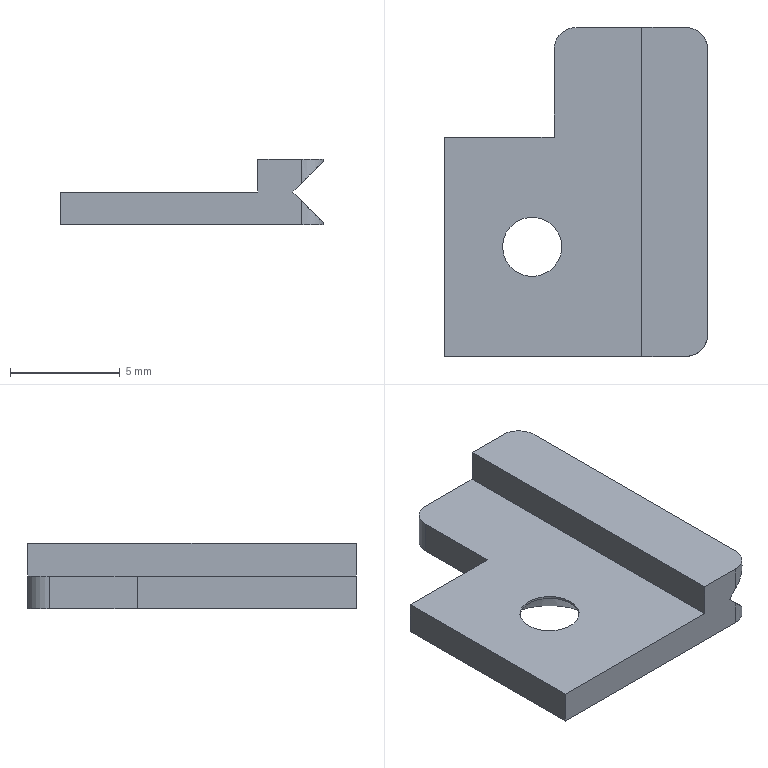Part | NX | features BREP 1 | 1 solid | 22 faces | box 12 x 15 x 3 mm | volume 250.226 mm3 | plane 13 | cylinder 7 | cone 2 | commonest cylinder face diameters 2 x5 2.7 x2
STEP:
#1=CARTESIAN_POINT('',(3.,7.5,3.));
#2=VERTEX_POINT('',#1);
#3=CARTESIAN_POINT('',(3.,7.5,1.5));
#4=VERTEX_POINT('',#3);
#5=CARTESIAN_POINT('',(3.,7.5,3.));
#6=DIRECTION('',(0.,0.,-1.));
#7=VECTOR('',#6,1000.);
#8=LINE('',#5,#7);
#9=EDGE_CURVE('',#2,#4,#8,.T.);
#10=ORIENTED_EDGE('',*,*,#9,.T.);
#11=CARTESIAN_POINT('',(3.,-7.5,1.5));
#12=VERTEX_POINT('',#11);
#13=CARTESIAN_POINT('',(3.,-7.5,1.5));
#14=DIRECTION('',(0.,1.,0.));
#15=VECTOR('',#14,1000.);
#16=LINE('',#13,#15);
#17=EDGE_CURVE('',#12,#4,#16,.T.);
#18=ORIENTED_EDGE('',*,*,#17,.F.);
#19=CARTESIAN_POINT('',(3.,-7.5,3.));
#20=VERTEX_POINT('',#19);
#21=CARTESIAN_POINT('',(3.,-7.5,3.));
#22=DIRECTION('',(0.,0.,-1.));
#23=VECTOR('',#22,1000.);
#24=LINE('',#21,#23);
#25=EDGE_CURVE('',#20,#12,#24,.T.);
#26=ORIENTED_EDGE('',*,*,#25,.F.);
#27=CARTESIAN_POINT('',(3.,-7.5,3.));
#28=DIRECTION('',(0.,1.,0.));
#29=VECTOR('',#28,1000.);
#30=LINE('',#27,#29);
#31=EDGE_CURVE('',#20,#2,#30,.T.);
#32=ORIENTED_EDGE('',*,*,#31,.T.);
#33=EDGE_LOOP('',(#10,#18,#26,#32));
#34=FACE_BOUND('',#33,.T.);
#35=CARTESIAN_POINT('',(3.,-7.5,3.));
#36=DIRECTION('',(1.,0.,0.));
#37=DIRECTION('',(0.,0.,-1.));
#38=AXIS2_PLACEMENT_3D('',#35,#36,#37);
#39=PLANE('',#38);
#40=ADVANCED_FACE('',(#34),#39,.F.);
#41=CARTESIAN_POINT('',(-6.,-7.5,1.5));
#42=VERTEX_POINT('',#41);
#43=CARTESIAN_POINT('',(-6.,2.5,1.5));
#44=VERTEX_POINT('',#43);
#45=CARTESIAN_POINT('',(-6.,-7.5,1.5));
#46=DIRECTION('',(0.,1.,0.));
#47=VECTOR('',#46,1000.);
#48=LINE('',#45,#47);
#49=EDGE_CURVE('',#42,#44,#48,.T.);
#50=ORIENTED_EDGE('',*,*,#49,.F.);
#51=CARTESIAN_POINT('',(-6.,-7.5,1.5));
#52=DIRECTION('',(-1.,0.,0.));
#53=VECTOR('',#52,1000.);
#54=LINE('',#51,#53);
#55=EDGE_CURVE('',#12,#42,#54,.T.);
#56=ORIENTED_EDGE('',*,*,#55,.F.);
#57=ORIENTED_EDGE('',*,*,#17,.T.);
#58=CARTESIAN_POINT('',(0.,7.5,1.5));
#59=VERTEX_POINT('',#58);
#60=CARTESIAN_POINT('',(-6.,7.5,1.5));
#61=DIRECTION('',(-1.,0.,0.));
#62=VECTOR('',#61,1000.);
#63=LINE('',#60,#62);
#64=EDGE_CURVE('',#4,#59,#63,.T.);
#65=ORIENTED_EDGE('',*,*,#64,.T.);
#66=CARTESIAN_POINT('',(-1.,6.5,1.5));
#67=VERTEX_POINT('',#66);
#68=CARTESIAN_POINT('',(0.,6.5,1.5));
#69=DIRECTION('',(0.,0.,1.));
#70=DIRECTION('',(-1.,0.,0.));
#71=AXIS2_PLACEMENT_3D('',#68,#69,#70);
#72=CIRCLE('',#71,1.);
#73=EDGE_CURVE('',#59,#67,#72,.T.);
#74=ORIENTED_EDGE('',*,*,#73,.T.);
#75=CARTESIAN_POINT('',(-1.,2.5,1.5));
#76=VERTEX_POINT('',#75);
#77=CARTESIAN_POINT('',(-1.,7.5,1.5));
#78=DIRECTION('',(0.,1.,0.));
#79=VECTOR('',#78,1000.);
#80=LINE('',#77,#79);
#81=EDGE_CURVE('',#76,#67,#80,.T.);
#82=ORIENTED_EDGE('',*,*,#81,.F.);
#83=CARTESIAN_POINT('',(-6.,2.5,1.5));
#84=DIRECTION('',(1.,0.,0.));
#85=VECTOR('',#84,1000.);
#86=LINE('',#83,#85);
#87=EDGE_CURVE('',#44,#76,#86,.T.);
#88=ORIENTED_EDGE('',*,*,#87,.F.);
#89=EDGE_LOOP('',(#50,#56,#57,#65,#74,#82,#88));
#90=FACE_BOUND('',#89,.T.);
#91=CARTESIAN_POINT('',(-3.35,-2.5,1.5));
#92=VERTEX_POINT('',#91);
#93=CARTESIAN_POINT('',(-0.65,-2.5,1.5));
#94=VERTEX_POINT('',#93);
#95=CARTESIAN_POINT('',(-2.,-2.5,1.5));
#96=DIRECTION('',(0.,0.,1.));
#97=DIRECTION('',(-1.,0.,0.));
#98=AXIS2_PLACEMENT_3D('',#95,#96,#97);
#99=CIRCLE('',#98,1.35);
#100=EDGE_CURVE('',#92,#94,#99,.T.);
#101=ORIENTED_EDGE('',*,*,#100,.F.);
#102=CARTESIAN_POINT('',(-2.,-2.5,1.5));
#103=DIRECTION('',(0.,0.,1.));
#104=DIRECTION('',(-1.,0.,0.));
#105=AXIS2_PLACEMENT_3D('',#102,#103,#104);
#106=CIRCLE('',#105,1.35);
#107=EDGE_CURVE('',#94,#92,#106,.T.);
#108=ORIENTED_EDGE('',*,*,#107,.F.);
#109=EDGE_LOOP('',(#101,#108));
#110=FACE_BOUND('',#109,.T.);
#111=CARTESIAN_POINT('',(-6.,-7.5,1.5));
#112=DIRECTION('',(0.,0.,-1.));
#113=DIRECTION('',(-1.,0.,0.));
#114=AXIS2_PLACEMENT_3D('',#111,#112,#113);
#115=PLANE('',#114);
#116=ADVANCED_FACE('',(#90,#110),#115,.F.);
#117=CARTESIAN_POINT('',(-0.65,-2.5,1.4));
#118=VERTEX_POINT('',#117);
#119=CARTESIAN_POINT('',(0.75,-2.5,0.));
#120=VERTEX_POINT('',#119);
#121=CARTESIAN_POINT('',(0.75,-2.5,0.));
#122=DIRECTION('',(0.7071,0.,-0.7071));
#123=VECTOR('',#122,1000.);
#124=LINE('',#121,#123);
#125=EDGE_CURVE('',#118,#120,#124,.T.);
#126=ORIENTED_EDGE('',*,*,#125,.F.);
#127=CARTESIAN_POINT('',(-3.35,-2.5,1.4));
#128=VERTEX_POINT('',#127);
#129=CARTESIAN_POINT('',(-2.,-2.5,1.4));
#130=DIRECTION('',(0.,0.,-1.));
#131=DIRECTION('',(-1.,0.,0.));
#132=AXIS2_PLACEMENT_3D('',#129,#130,#131);
#133=CIRCLE('',#132,1.35);
#134=EDGE_CURVE('',#128,#118,#133,.T.);
#135=ORIENTED_EDGE('',*,*,#134,.F.);
#136=CARTESIAN_POINT('',(-4.75,-2.5,0.));
#137=VERTEX_POINT('',#136);
#138=CARTESIAN_POINT('',(-4.75,-2.5,0.));
#139=DIRECTION('',(-0.7071,0.,-0.7071));
#140=VECTOR('',#139,1000.);
#141=LINE('',#138,#140);
#142=EDGE_CURVE('',#128,#137,#141,.T.);
#143=ORIENTED_EDGE('',*,*,#142,.T.);
#144=CARTESIAN_POINT('',(-2.,-2.5,0.));
#145=DIRECTION('',(0.,0.,-1.));
#146=DIRECTION('',(-1.,0.,0.));
#147=AXIS2_PLACEMENT_3D('',#144,#145,#146);
#148=CIRCLE('',#147,2.75);
#149=EDGE_CURVE('',#137,#120,#148,.T.);
#150=ORIENTED_EDGE('',*,*,#149,.T.);
#151=EDGE_LOOP('',(#126,#135,#143,#150));
#152=FACE_BOUND('',#151,.T.);
#153=CARTESIAN_POINT('',(-2.,-2.5,0.));
#154=DIRECTION('',(0.,0.,-1.));
#155=DIRECTION('',(-1.,0.,0.));
#156=AXIS2_PLACEMENT_3D('',#153,#154,#155);
#157=CONICAL_SURFACE('',#156,2.75,0.7854);
#158=ADVANCED_FACE('',(#152),#157,.F.);
#159=CARTESIAN_POINT('',(-0.65,-2.5,0.));
#160=DIRECTION('',(0.,0.,-1.));
#161=VECTOR('',#160,1000.);
#162=LINE('',#159,#161);
#163=EDGE_CURVE('',#94,#118,#162,.T.);
#164=ORIENTED_EDGE('',*,*,#163,.F.);
#165=ORIENTED_EDGE('',*,*,#107,.T.);
#166=CARTESIAN_POINT('',(-3.35,-2.5,0.));
#167=DIRECTION('',(0.,0.,-1.));
#168=VECTOR('',#167,1000.);
#169=LINE('',#166,#168);
#170=EDGE_CURVE('',#92,#128,#169,.T.);
#171=ORIENTED_EDGE('',*,*,#170,.T.);
#172=ORIENTED_EDGE('',*,*,#134,.T.);
#173=EDGE_LOOP('',(#164,#165,#171,#172));
#174=FACE_BOUND('',#173,.T.);
#175=CARTESIAN_POINT('',(-2.,-2.5,0.));
#176=DIRECTION('',(0.,0.,-1.));
#177=DIRECTION('',(-1.,0.,0.));
#178=AXIS2_PLACEMENT_3D('',#175,#176,#177);
#179=CYLINDRICAL_SURFACE('',#178,1.35);
#180=ADVANCED_FACE('',(#174),#179,.F.);
#181=CARTESIAN_POINT('',(5.,-7.5,1.1));
#182=VERTEX_POINT('',#181);
#183=CARTESIAN_POINT('',(6.,-6.5,0.1));
#184=VERTEX_POINT('',#183);
#185=CARTESIAN_POINT('',(5.,-7.5,1.1));
#186=CARTESIAN_POINT('',(5.586,-7.5,0.5142));
#187=CARTESIAN_POINT('',(6.,-7.086,0.1));
#188=CARTESIAN_POINT('',(6.,-6.5,0.1));
#189=(BOUNDED_CURVE()B_SPLINE_CURVE(3,(#185,#186,#187,#188),.UNSPECIFIED.,.F.,.F.)B_SPLINE_CURVE_WITH_KNOTS((4,4),(4.712,6.283),.UNSPECIFIED.)CURVE()GEOMETRIC_REPRESENTATION_ITEM()RATIONAL_B_SPLINE_CURVE((1.,0.8047,0.8047,1.))REPRESENTATION_ITEM(''));
#190=EDGE_CURVE('',#182,#184,#189,.T.);
#191=ORIENTED_EDGE('',*,*,#190,.T.);
#192=CARTESIAN_POINT('',(6.,6.5,0.1));
#193=VERTEX_POINT('',#192);
#194=CARTESIAN_POINT('',(6.,-12.5,0.1));
#195=DIRECTION('',(0.,1.,0.));
#196=VECTOR('',#195,1000.);
#197=LINE('',#194,#196);
#198=EDGE_CURVE('',#184,#193,#197,.T.);
#199=ORIENTED_EDGE('',*,*,#198,.T.);
#200=CARTESIAN_POINT('',(5.,7.5,1.1));
#201=VERTEX_POINT('',#200);
#202=CARTESIAN_POINT('',(6.,6.5,0.1));
#203=CARTESIAN_POINT('',(6.,7.086,0.1));
#204=CARTESIAN_POINT('',(5.586,7.5,0.5142));
#205=CARTESIAN_POINT('',(5.,7.5,1.1));
#206=(BOUNDED_CURVE()B_SPLINE_CURVE(3,(#202,#203,#204,#205),.UNSPECIFIED.,.F.,.F.)B_SPLINE_CURVE_WITH_KNOTS((4,4),(0.,1.571),.UNSPECIFIED.)CURVE()GEOMETRIC_REPRESENTATION_ITEM()RATIONAL_B_SPLINE_CURVE((1.,0.8047,0.8047,1.))REPRESENTATION_ITEM(''));
#207=EDGE_CURVE('',#193,#201,#206,.T.);
#208=ORIENTED_EDGE('',*,*,#207,.T.);
#209=CARTESIAN_POINT('',(4.6,7.5,1.5));
#210=VERTEX_POINT('',#209);
#211=CARTESIAN_POINT('',(4.6,7.5,1.5));
#212=DIRECTION('',(-0.7071,0.,0.7071));
#213=VECTOR('',#212,1000.);
#214=LINE('',#211,#213);
#215=EDGE_CURVE('',#201,#210,#214,.T.);
#216=ORIENTED_EDGE('',*,*,#215,.T.);
#217=CARTESIAN_POINT('',(4.6,-7.5,1.5));
#218=VERTEX_POINT('',#217);
#219=CARTESIAN_POINT('',(4.6,-12.5,1.5));
#220=DIRECTION('',(0.,1.,0.));
#221=VECTOR('',#220,1000.);
#222=LINE('',#219,#221);
#223=EDGE_CURVE('',#218,#210,#222,.T.);
#224=ORIENTED_EDGE('',*,*,#223,.F.);
#225=CARTESIAN_POINT('',(-1.45,-7.5,7.55));
#226=DIRECTION('',(-0.7071,0.,0.7071));
#227=VECTOR('',#226,1000.);
#228=LINE('',#225,#227);
#229=EDGE_CURVE('',#182,#218,#228,.T.);
#230=ORIENTED_EDGE('',*,*,#229,.F.);
#231=EDGE_LOOP('',(#191,#199,#208,#216,#224,#230));
#232=FACE_BOUND('',#231,.T.);
#233=CARTESIAN_POINT('',(4.6,-12.5,1.5));
#234=DIRECTION('',(-0.7071,0.,-0.7071));
#235=DIRECTION('',(-0.7071,0.,0.7071));
#236=AXIS2_PLACEMENT_3D('',#233,#234,#235);
#237=PLANE('',#236);
#238=ADVANCED_FACE('',(#232),#237,.F.);
#239=ORIENTED_EDGE('',*,*,#223,.T.);
#240=CARTESIAN_POINT('',(5.,7.5,1.9));
#241=VERTEX_POINT('',#240);
#242=CARTESIAN_POINT('',(6.,7.5,2.9));
#243=DIRECTION('',(0.7071,0.,0.7071));
#244=VECTOR('',#243,1000.);
#245=LINE('',#242,#244);
#246=EDGE_CURVE('',#210,#241,#245,.T.);
#247=ORIENTED_EDGE('',*,*,#246,.T.);
#248=CARTESIAN_POINT('',(6.,6.5,2.9));
#249=VERTEX_POINT('',#248);
#250=CARTESIAN_POINT('',(5.,7.5,1.9));
#251=CARTESIAN_POINT('',(5.586,7.5,2.486));
#252=CARTESIAN_POINT('',(6.,7.086,2.9));
#253=CARTESIAN_POINT('',(6.,6.5,2.9));
#254=(BOUNDED_CURVE()B_SPLINE_CURVE(3,(#250,#251,#252,#253),.UNSPECIFIED.,.F.,.F.)B_SPLINE_CURVE_WITH_KNOTS((4,4),(1.571,3.142),.UNSPECIFIED.)CURVE()GEOMETRIC_REPRESENTATION_ITEM()RATIONAL_B_SPLINE_CURVE((1.,0.8047,0.8047,1.))REPRESENTATION_ITEM(''));
#255=EDGE_CURVE('',#241,#249,#254,.T.);
#256=ORIENTED_EDGE('',*,*,#255,.T.);
#257=CARTESIAN_POINT('',(6.,-6.5,2.9));
#258=VERTEX_POINT('',#257);
#259=CARTESIAN_POINT('',(6.,-12.5,2.9));
#260=DIRECTION('',(0.,1.,0.));
#261=VECTOR('',#260,1000.);
#262=LINE('',#259,#261);
#263=EDGE_CURVE('',#258,#249,#262,.T.);
#264=ORIENTED_EDGE('',*,*,#263,.F.);
#265=CARTESIAN_POINT('',(5.,-7.5,1.9));
#266=VERTEX_POINT('',#265);
#267=CARTESIAN_POINT('',(6.,-6.5,2.9));
#268=CARTESIAN_POINT('',(6.,-7.086,2.9));
#269=CARTESIAN_POINT('',(5.586,-7.5,2.486));
#270=CARTESIAN_POINT('',(5.,-7.5,1.9));
#271=(BOUNDED_CURVE()B_SPLINE_CURVE(3,(#267,#268,#269,#270),.UNSPECIFIED.,.F.,.F.)B_SPLINE_CURVE_WITH_KNOTS((4,4),(3.142,4.712),.UNSPECIFIED.)CURVE()GEOMETRIC_REPRESENTATION_ITEM()RATIONAL_B_SPLINE_CURVE((1.,0.8047,0.8047,1.))REPRESENTATION_ITEM(''));
#272=EDGE_CURVE('',#258,#266,#271,.T.);
#273=ORIENTED_EDGE('',*,*,#272,.T.);
#274=CARTESIAN_POINT('',(0.05,-7.5,-3.05));
#275=DIRECTION('',(0.7071,0.,0.7071));
#276=VECTOR('',#275,1000.);
#277=LINE('',#274,#276);
#278=EDGE_CURVE('',#218,#266,#277,.T.);
#279=ORIENTED_EDGE('',*,*,#278,.F.);
#280=EDGE_LOOP('',(#239,#247,#256,#264,#273,#279));
#281=FACE_BOUND('',#280,.T.);
#282=CARTESIAN_POINT('',(6.,-12.5,2.9));
#283=DIRECTION('',(-0.7071,0.,0.7071));
#284=DIRECTION('',(0.7071,0.,0.7071));
#285=AXIS2_PLACEMENT_3D('',#282,#283,#284);
#286=PLANE('',#285);
#287=ADVANCED_FACE('',(#281),#286,.F.);
#288=ORIENTED_EDGE('',*,*,#207,.F.);
#289=CARTESIAN_POINT('',(6.,6.5,0.));
#290=VERTEX_POINT('',#289);
#291=CARTESIAN_POINT('',(6.,6.5,3.));
#292=DIRECTION('',(0.,0.,1.));
#293=VECTOR('',#292,1000.);
#294=LINE('',#291,#293);
#295=EDGE_CURVE('',#290,#193,#294,.T.);
#296=ORIENTED_EDGE('',*,*,#295,.F.);
#297=CARTESIAN_POINT('',(5.,7.5,0.));
#298=VERTEX_POINT('',#297);
#299=CARTESIAN_POINT('',(5.,6.5,0.));
#300=DIRECTION('',(0.,0.,-1.));
#301=DIRECTION('',(-1.,0.,0.));
#302=AXIS2_PLACEMENT_3D('',#299,#300,#301);
#303=CIRCLE('',#302,1.);
#304=EDGE_CURVE('',#298,#290,#303,.T.);
#305=ORIENTED_EDGE('',*,*,#304,.F.);
#306=CARTESIAN_POINT('',(5.,7.5,3.));
#307=DIRECTION('',(0.,0.,-1.));
#308=VECTOR('',#307,1000.);
#309=LINE('',#306,#308);
#310=EDGE_CURVE('',#201,#298,#309,.T.);
#311=ORIENTED_EDGE('',*,*,#310,.F.);
#312=EDGE_LOOP('',(#288,#296,#305,#311));
#313=FACE_BOUND('',#312,.T.);
#314=CARTESIAN_POINT('',(5.,6.5,3.));
#315=DIRECTION('',(0.,0.,-1.));
#316=DIRECTION('',(-1.,0.,0.));
#317=AXIS2_PLACEMENT_3D('',#314,#315,#316);
#318=CYLINDRICAL_SURFACE('',#317,1.);
#319=ADVANCED_FACE('',(#313),#318,.T.);
#320=ORIENTED_EDGE('',*,*,#190,.F.);
#321=CARTESIAN_POINT('',(5.,-7.5,0.));
#322=VERTEX_POINT('',#321);
#323=CARTESIAN_POINT('',(5.,-7.5,3.));
#324=DIRECTION('',(0.,0.,1.));
#325=VECTOR('',#324,1000.);
#326=LINE('',#323,#325);
#327=EDGE_CURVE('',#322,#182,#326,.T.);
#328=ORIENTED_EDGE('',*,*,#327,.F.);
#329=CARTESIAN_POINT('',(6.,-6.5,0.));
#330=VERTEX_POINT('',#329);
#331=CARTESIAN_POINT('',(5.,-6.5,0.));
#332=DIRECTION('',(0.,0.,-1.));
#333=DIRECTION('',(-1.,0.,0.));
#334=AXIS2_PLACEMENT_3D('',#331,#332,#333);
#335=CIRCLE('',#334,1.);
#336=EDGE_CURVE('',#330,#322,#335,.T.);
#337=ORIENTED_EDGE('',*,*,#336,.F.);
#338=CARTESIAN_POINT('',(6.,-6.5,3.));
#339=DIRECTION('',(0.,0.,-1.));
#340=VECTOR('',#339,1000.);
#341=LINE('',#338,#340);
#342=EDGE_CURVE('',#184,#330,#341,.T.);
#343=ORIENTED_EDGE('',*,*,#342,.F.);
#344=EDGE_LOOP('',(#320,#328,#337,#343));
#345=FACE_BOUND('',#344,.T.);
#346=CARTESIAN_POINT('',(5.,-6.5,3.));
#347=DIRECTION('',(0.,0.,-1.));
#348=DIRECTION('',(-1.,0.,0.));
#349=AXIS2_PLACEMENT_3D('',#346,#347,#348);
#350=CYLINDRICAL_SURFACE('',#349,1.);
#351=ADVANCED_FACE('',(#345),#350,.T.);
#352=ORIENTED_EDGE('',*,*,#73,.F.);
#353=CARTESIAN_POINT('',(0.,7.5,0.));
#354=VERTEX_POINT('',#353);
#355=CARTESIAN_POINT('',(0.,7.5,3.));
#356=DIRECTION('',(0.,0.,1.));
#357=VECTOR('',#356,1000.);
#358=LINE('',#355,#357);
#359=EDGE_CURVE('',#354,#59,#358,.T.);
#360=ORIENTED_EDGE('',*,*,#359,.F.);
#361=CARTESIAN_POINT('',(-1.,6.5,0.));
#362=VERTEX_POINT('',#361);
#363=CARTESIAN_POINT('',(0.,6.5,0.));
#364=DIRECTION('',(0.,0.,-1.));
#365=DIRECTION('',(-1.,0.,0.));
#366=AXIS2_PLACEMENT_3D('',#363,#364,#365);
#367=CIRCLE('',#366,1.);
#368=EDGE_CURVE('',#362,#354,#367,.T.);
#369=ORIENTED_EDGE('',*,*,#368,.F.);
#370=CARTESIAN_POINT('',(-1.,6.5,3.));
#371=DIRECTION('',(0.,0.,-1.));
#372=VECTOR('',#371,1000.);
#373=LINE('',#370,#372);
#374=EDGE_CURVE('',#67,#362,#373,.T.);
#375=ORIENTED_EDGE('',*,*,#374,.F.);
#376=EDGE_LOOP('',(#352,#360,#369,#375));
#377=FACE_BOUND('',#376,.T.);
#378=CARTESIAN_POINT('',(0.,6.5,3.));
#379=DIRECTION('',(0.,0.,-1.));
#380=DIRECTION('',(-1.,0.,0.));
#381=AXIS2_PLACEMENT_3D('',#378,#379,#380);
#382=CYLINDRICAL_SURFACE('',#381,1.);
#383=ADVANCED_FACE('',(#377),#382,.T.);
#384=CARTESIAN_POINT('',(-1.,2.5,0.));
#385=VERTEX_POINT('',#384);
#386=CARTESIAN_POINT('',(-1.,2.5,3.));
#387=DIRECTION('',(0.,0.,-1.));
#388=VECTOR('',#387,1000.);
#389=LINE('',#386,#388);
#390=EDGE_CURVE('',#76,#385,#389,.T.);
#391=ORIENTED_EDGE('',*,*,#390,.F.);
#392=ORIENTED_EDGE('',*,*,#81,.T.);
#393=ORIENTED_EDGE('',*,*,#374,.T.);
#394=CARTESIAN_POINT('',(-1.,7.5,0.));
#395=DIRECTION('',(0.,-1.,0.));
#396=VECTOR('',#395,1000.);
#397=LINE('',#394,#396);
#398=EDGE_CURVE('',#362,#385,#397,.T.);
#399=ORIENTED_EDGE('',*,*,#398,.T.);
#400=EDGE_LOOP('',(#391,#392,#393,#399));
#401=FACE_BOUND('',#400,.T.);
#402=CARTESIAN_POINT('',(-1.,7.5,3.));
#403=DIRECTION('',(1.,0.,0.));
#404=DIRECTION('',(0.,1.,0.));
#405=AXIS2_PLACEMENT_3D('',#402,#403,#404);
#406=PLANE('',#405);
#407=ADVANCED_FACE('',(#401),#406,.F.);
#408=CARTESIAN_POINT('',(-6.,2.5,0.));
#409=VERTEX_POINT('',#408);
#410=CARTESIAN_POINT('',(-6.,2.5,3.));
#411=DIRECTION('',(0.,0.,-1.));
#412=VECTOR('',#411,1000.);
#413=LINE('',#410,#412);
#414=EDGE_CURVE('',#44,#409,#413,.T.);
#415=ORIENTED_EDGE('',*,*,#414,.F.);
#416=ORIENTED_EDGE('',*,*,#87,.T.);
#417=ORIENTED_EDGE('',*,*,#390,.T.);
#418=CARTESIAN_POINT('',(-6.,2.5,0.));
#419=DIRECTION('',(-1.,0.,0.));
#420=VECTOR('',#419,1000.);
#421=LINE('',#418,#420);
#422=EDGE_CURVE('',#385,#409,#421,.T.);
#423=ORIENTED_EDGE('',*,*,#422,.T.);
#424=EDGE_LOOP('',(#415,#416,#417,#423));
#425=FACE_BOUND('',#424,.T.);
#426=CARTESIAN_POINT('',(-6.,2.5,3.));
#427=DIRECTION('',(0.,-1.,0.));
#428=DIRECTION('',(1.,0.,0.));
#429=AXIS2_PLACEMENT_3D('',#426,#427,#428);
#430=PLANE('',#429);
#431=ADVANCED_FACE('',(#425),#430,.F.);
#432=ORIENTED_EDGE('',*,*,#398,.F.);
#433=ORIENTED_EDGE('',*,*,#368,.T.);
#434=CARTESIAN_POINT('',(-6.,7.5,0.));
#435=DIRECTION('',(-1.,0.,0.));
#436=VECTOR('',#435,1000.);
#437=LINE('',#434,#436);
#438=EDGE_CURVE('',#298,#354,#437,.T.);
#439=ORIENTED_EDGE('',*,*,#438,.F.);
#440=ORIENTED_EDGE('',*,*,#304,.T.);
#441=CARTESIAN_POINT('',(6.,-7.5,0.));
#442=DIRECTION('',(0.,1.,0.));
#443=VECTOR('',#442,1000.);
#444=LINE('',#441,#443);
#445=EDGE_CURVE('',#330,#290,#444,.T.);
#446=ORIENTED_EDGE('',*,*,#445,.F.);
#447=ORIENTED_EDGE('',*,*,#336,.T.);
#448=CARTESIAN_POINT('',(-6.,-7.5,0.));
#449=VERTEX_POINT('',#448);
#450=CARTESIAN_POINT('',(-6.,-7.5,0.));
#451=DIRECTION('',(1.,0.,0.));
#452=VECTOR('',#451,1000.);
#453=LINE('',#450,#452);
#454=EDGE_CURVE('',#449,#322,#453,.T.);
#455=ORIENTED_EDGE('',*,*,#454,.F.);
#456=CARTESIAN_POINT('',(-6.,-7.5,0.));
#457=DIRECTION('',(0.,-1.,0.));
#458=VECTOR('',#457,1000.);
#459=LINE('',#456,#458);
#460=EDGE_CURVE('',#409,#449,#459,.T.);
#461=ORIENTED_EDGE('',*,*,#460,.F.);
#462=ORIENTED_EDGE('',*,*,#422,.F.);
#463=EDGE_LOOP('',(#432,#433,#439,#440,#446,#447,#455,#461,#462));
#464=FACE_BOUND('',#463,.T.);
#465=ORIENTED_EDGE('',*,*,#149,.F.);
#466=CARTESIAN_POINT('',(-2.,-2.5,0.));
#467=DIRECTION('',(0.,0.,-1.));
#468=DIRECTION('',(-1.,0.,0.));
#469=AXIS2_PLACEMENT_3D('',#466,#467,#468);
#470=CIRCLE('',#469,2.75);
#471=EDGE_CURVE('',#120,#137,#470,.T.);
#472=ORIENTED_EDGE('',*,*,#471,.F.);
#473=EDGE_LOOP('',(#465,#472));
#474=FACE_BOUND('',#473,.T.);
#475=CARTESIAN_POINT('',(0.,0.,0.));
#476=DIRECTION('',(0.,0.,-1.));
#477=DIRECTION('',(-1.,0.,0.));
#478=AXIS2_PLACEMENT_3D('',#475,#476,#477);
#479=PLANE('',#478);
#480=ADVANCED_FACE('',(#464,#474),#479,.T.);
#481=CARTESIAN_POINT('',(5.,7.5,3.));
#482=VERTEX_POINT('',#481);
#483=CARTESIAN_POINT('',(-6.,7.5,3.));
#484=DIRECTION('',(-1.,0.,0.));
#485=VECTOR('',#484,1000.);
#486=LINE('',#483,#485);
#487=EDGE_CURVE('',#482,#2,#486,.T.);
#488=ORIENTED_EDGE('',*,*,#487,.T.);
#489=ORIENTED_EDGE('',*,*,#31,.F.);
#490=CARTESIAN_POINT('',(5.,-7.5,3.));
#491=VERTEX_POINT('',#490);
#492=CARTESIAN_POINT('',(-6.,-7.5,3.));
#493=DIRECTION('',(1.,0.,0.));
#494=VECTOR('',#493,1000.);
#495=LINE('',#492,#494);
#496=EDGE_CURVE('',#20,#491,#495,.T.);
#497=ORIENTED_EDGE('',*,*,#496,.T.);
#498=CARTESIAN_POINT('',(6.,-6.5,3.));
#499=VERTEX_POINT('',#498);
#500=CARTESIAN_POINT('',(5.,-6.5,3.));
#501=DIRECTION('',(0.,0.,1.));
#502=DIRECTION('',(-1.,0.,0.));
#503=AXIS2_PLACEMENT_3D('',#500,#501,#502);
#504=CIRCLE('',#503,1.);
#505=EDGE_CURVE('',#491,#499,#504,.T.);
#506=ORIENTED_EDGE('',*,*,#505,.T.);
#507=CARTESIAN_POINT('',(6.,6.5,3.));
#508=VERTEX_POINT('',#507);
#509=CARTESIAN_POINT('',(6.,-7.5,3.));
#510=DIRECTION('',(0.,1.,0.));
#511=VECTOR('',#510,1000.);
#512=LINE('',#509,#511);
#513=EDGE_CURVE('',#499,#508,#512,.T.);
#514=ORIENTED_EDGE('',*,*,#513,.T.);
#515=CARTESIAN_POINT('',(5.,6.5,3.));
#516=DIRECTION('',(0.,0.,1.));
#517=DIRECTION('',(-1.,0.,0.));
#518=AXIS2_PLACEMENT_3D('',#515,#516,#517);
#519=CIRCLE('',#518,1.);
#520=EDGE_CURVE('',#508,#482,#519,.T.);
#521=ORIENTED_EDGE('',*,*,#520,.T.);
#522=EDGE_LOOP('',(#488,#489,#497,#506,#514,#521));
#523=FACE_BOUND('',#522,.T.);
#524=CARTESIAN_POINT('',(0.,0.,3.));
#525=DIRECTION('',(0.,0.,-1.));
#526=DIRECTION('',(-1.,0.,0.));
#527=AXIS2_PLACEMENT_3D('',#524,#525,#526);
#528=PLANE('',#527);
#529=ADVANCED_FACE('',(#523),#528,.F.);
#530=ORIENTED_EDGE('',*,*,#25,.T.);
#531=ORIENTED_EDGE('',*,*,#55,.T.);
#532=CARTESIAN_POINT('',(-6.,-7.5,3.));
#533=DIRECTION('',(0.,0.,-1.));
#534=VECTOR('',#533,1000.);
#535=LINE('',#532,#534);
#536=EDGE_CURVE('',#42,#449,#535,.T.);
#537=ORIENTED_EDGE('',*,*,#536,.T.);
#538=ORIENTED_EDGE('',*,*,#454,.T.);
#539=ORIENTED_EDGE('',*,*,#327,.T.);
#540=ORIENTED_EDGE('',*,*,#229,.T.);
#541=ORIENTED_EDGE('',*,*,#278,.T.);
#542=CARTESIAN_POINT('',(5.,-7.5,3.));
#543=DIRECTION('',(0.,0.,1.));
#544=VECTOR('',#543,1000.);
#545=LINE('',#542,#544);
#546=EDGE_CURVE('',#266,#491,#545,.T.);
#547=ORIENTED_EDGE('',*,*,#546,.T.);
#548=ORIENTED_EDGE('',*,*,#496,.F.);
#549=EDGE_LOOP('',(#530,#531,#537,#538,#539,#540,#541,#547,#548));
#550=FACE_BOUND('',#549,.T.);
#551=CARTESIAN_POINT('',(-6.,-7.5,3.));
#552=DIRECTION('',(0.,1.,0.));
#553=DIRECTION('',(0.,0.,1.));
#554=AXIS2_PLACEMENT_3D('',#551,#552,#553);
#555=PLANE('',#554);
#556=ADVANCED_FACE('',(#550),#555,.F.);
#557=ORIENTED_EDGE('',*,*,#536,.F.);
#558=ORIENTED_EDGE('',*,*,#49,.T.);
#559=ORIENTED_EDGE('',*,*,#414,.T.);
#560=ORIENTED_EDGE('',*,*,#460,.T.);
#561=EDGE_LOOP('',(#557,#558,#559,#560));
#562=FACE_BOUND('',#561,.T.);
#563=CARTESIAN_POINT('',(-6.,-7.5,3.));
#564=DIRECTION('',(1.,0.,0.));
#565=DIRECTION('',(0.,0.,-1.));
#566=AXIS2_PLACEMENT_3D('',#563,#564,#565);
#567=PLANE('',#566);
#568=ADVANCED_FACE('',(#562),#567,.F.);
#569=ORIENTED_EDGE('',*,*,#359,.T.);
#570=ORIENTED_EDGE('',*,*,#64,.F.);
#571=ORIENTED_EDGE('',*,*,#9,.F.);
#572=ORIENTED_EDGE('',*,*,#487,.F.);
#573=CARTESIAN_POINT('',(5.,7.5,3.));
#574=DIRECTION('',(0.,0.,-1.));
#575=VECTOR('',#574,1000.);
#576=LINE('',#573,#575);
#577=EDGE_CURVE('',#482,#241,#576,.T.);
#578=ORIENTED_EDGE('',*,*,#577,.T.);
#579=ORIENTED_EDGE('',*,*,#246,.F.);
#580=ORIENTED_EDGE('',*,*,#215,.F.);
#581=ORIENTED_EDGE('',*,*,#310,.T.);
#582=ORIENTED_EDGE('',*,*,#438,.T.);
#583=EDGE_LOOP('',(#569,#570,#571,#572,#578,#579,#580,#581,#582));
#584=FACE_BOUND('',#583,.T.);
#585=CARTESIAN_POINT('',(-6.,7.5,3.));
#586=DIRECTION('',(0.,-1.,0.));
#587=DIRECTION('',(0.,0.,-1.));
#588=AXIS2_PLACEMENT_3D('',#585,#586,#587);
#589=PLANE('',#588);
#590=ADVANCED_FACE('',(#584),#589,.F.);
#591=ORIENTED_EDGE('',*,*,#295,.T.);
#592=ORIENTED_EDGE('',*,*,#198,.F.);
#593=ORIENTED_EDGE('',*,*,#342,.T.);
#594=ORIENTED_EDGE('',*,*,#445,.T.);
#595=EDGE_LOOP('',(#591,#592,#593,#594));
#596=FACE_BOUND('',#595,.T.);
#597=CARTESIAN_POINT('',(6.,-7.5,3.));
#598=DIRECTION('',(-1.,0.,0.));
#599=DIRECTION('',(0.,0.,1.));
#600=AXIS2_PLACEMENT_3D('',#597,#598,#599);
#601=PLANE('',#600);
#602=ADVANCED_FACE('',(#596),#601,.F.);
#603=ORIENTED_EDGE('',*,*,#255,.F.);
#604=ORIENTED_EDGE('',*,*,#577,.F.);
#605=ORIENTED_EDGE('',*,*,#520,.F.);
#606=CARTESIAN_POINT('',(6.,6.5,3.));
#607=DIRECTION('',(0.,0.,1.));
#608=VECTOR('',#607,1000.);
#609=LINE('',#606,#608);
#610=EDGE_CURVE('',#249,#508,#609,.T.);
#611=ORIENTED_EDGE('',*,*,#610,.F.);
#612=EDGE_LOOP('',(#603,#604,#605,#611));
#613=FACE_BOUND('',#612,.T.);
#614=CARTESIAN_POINT('',(5.,6.5,3.));
#615=DIRECTION('',(0.,0.,-1.));
#616=DIRECTION('',(-1.,0.,0.));
#617=AXIS2_PLACEMENT_3D('',#614,#615,#616);
#618=CYLINDRICAL_SURFACE('',#617,1.);
#619=ADVANCED_FACE('',(#613),#618,.T.);
#620=ORIENTED_EDGE('',*,*,#272,.F.);
#621=CARTESIAN_POINT('',(6.,-6.5,3.));
#622=DIRECTION('',(0.,0.,-1.));
#623=VECTOR('',#622,1000.);
#624=LINE('',#621,#623);
#625=EDGE_CURVE('',#499,#258,#624,.T.);
#626=ORIENTED_EDGE('',*,*,#625,.F.);
#627=ORIENTED_EDGE('',*,*,#505,.F.);
#628=ORIENTED_EDGE('',*,*,#546,.F.);
#629=EDGE_LOOP('',(#620,#626,#627,#628));
#630=FACE_BOUND('',#629,.T.);
#631=CARTESIAN_POINT('',(5.,-6.5,3.));
#632=DIRECTION('',(0.,0.,-1.));
#633=DIRECTION('',(-1.,0.,0.));
#634=AXIS2_PLACEMENT_3D('',#631,#632,#633);
#635=CYLINDRICAL_SURFACE('',#634,1.);
#636=ADVANCED_FACE('',(#630),#635,.T.);
#637=ORIENTED_EDGE('',*,*,#625,.T.);
#638=ORIENTED_EDGE('',*,*,#263,.T.);
#639=ORIENTED_EDGE('',*,*,#610,.T.);
#640=ORIENTED_EDGE('',*,*,#513,.F.);
#641=EDGE_LOOP('',(#637,#638,#639,#640));
#642=FACE_BOUND('',#641,.T.);
#643=CARTESIAN_POINT('',(6.,-7.5,3.));
#644=DIRECTION('',(-1.,0.,0.));
#645=DIRECTION('',(0.,0.,1.));
#646=AXIS2_PLACEMENT_3D('',#643,#644,#645);
#647=PLANE('',#646);
#648=ADVANCED_FACE('',(#642),#647,.F.);
#649=ORIENTED_EDGE('',*,*,#100,.T.);
#650=ORIENTED_EDGE('',*,*,#163,.T.);
#651=CARTESIAN_POINT('',(-2.,-2.5,1.4));
#652=DIRECTION('',(0.,0.,-1.));
#653=DIRECTION('',(-1.,0.,0.));
#654=AXIS2_PLACEMENT_3D('',#651,#652,#653);
#655=CIRCLE('',#654,1.35);
#656=EDGE_CURVE('',#118,#128,#655,.T.);
#657=ORIENTED_EDGE('',*,*,#656,.T.);
#658=ORIENTED_EDGE('',*,*,#170,.F.);
#659=EDGE_LOOP('',(#649,#650,#657,#658));
#660=FACE_BOUND('',#659,.T.);
#661=CARTESIAN_POINT('',(-2.,-2.5,0.));
#662=DIRECTION('',(0.,0.,-1.));
#663=DIRECTION('',(-1.,0.,0.));
#664=AXIS2_PLACEMENT_3D('',#661,#662,#663);
#665=CYLINDRICAL_SURFACE('',#664,1.35);
#666=ADVANCED_FACE('',(#660),#665,.F.);
#667=ORIENTED_EDGE('',*,*,#656,.F.);
#668=ORIENTED_EDGE('',*,*,#125,.T.);
#669=ORIENTED_EDGE('',*,*,#471,.T.);
#670=ORIENTED_EDGE('',*,*,#142,.F.);
#671=EDGE_LOOP('',(#667,#668,#669,#670));
#672=FACE_BOUND('',#671,.T.);
#673=CARTESIAN_POINT('',(-2.,-2.5,0.));
#674=DIRECTION('',(0.,0.,-1.));
#675=DIRECTION('',(-1.,0.,0.));
#676=AXIS2_PLACEMENT_3D('',#673,#674,#675);
#677=CONICAL_SURFACE('',#676,2.75,0.7854);
#678=ADVANCED_FACE('',(#672),#677,.F.);
#679=CLOSED_SHELL('',(#40,#116,#158,#180,#238,#287,#319,#351,#383,#407,#431,#480,#529,#556,#568,#590,#602,#619,#636,#648,#666,#678));
#680=MANIFOLD_SOLID_BREP('',#679);
#681=(LENGTH_UNIT()NAMED_UNIT(*)SI_UNIT(.MILLI.,.METRE.));
#682=UNCERTAINTY_MEASURE_WITH_UNIT(LENGTH_MEASURE(0.00001),#681,'','');
#683=(NAMED_UNIT(*)PLANE_ANGLE_UNIT()SI_UNIT($,.RADIAN.));
#684=(NAMED_UNIT(*)SI_UNIT($,.STERADIAN.)SOLID_ANGLE_UNIT());
#685=(GEOMETRIC_REPRESENTATION_CONTEXT(3)GLOBAL_UNCERTAINTY_ASSIGNED_CONTEXT((#682))GLOBAL_UNIT_ASSIGNED_CONTEXT((#681,#683,#684))REPRESENTATION_CONTEXT('',''));
#686=ADVANCED_BREP_SHAPE_REPRESENTATION('',(#680),#685);